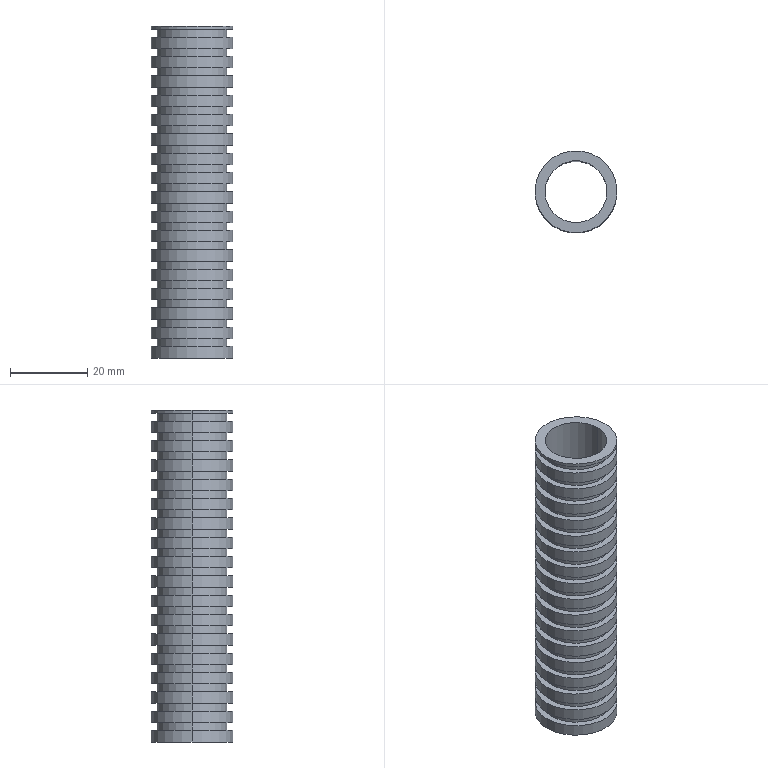Part | STEP file | P0177566_EZT_SCHUTZSCHLAUCH_MKR-16.5-PG-16_1 | 1 solid | 108 faces | box 21.2 x 21.2 x 85.851 mm | volume 9693 mm3 | cylinder 72 | plane 36 | commonest cylinder face diameters 21.2 x36 18 x34 16 x2